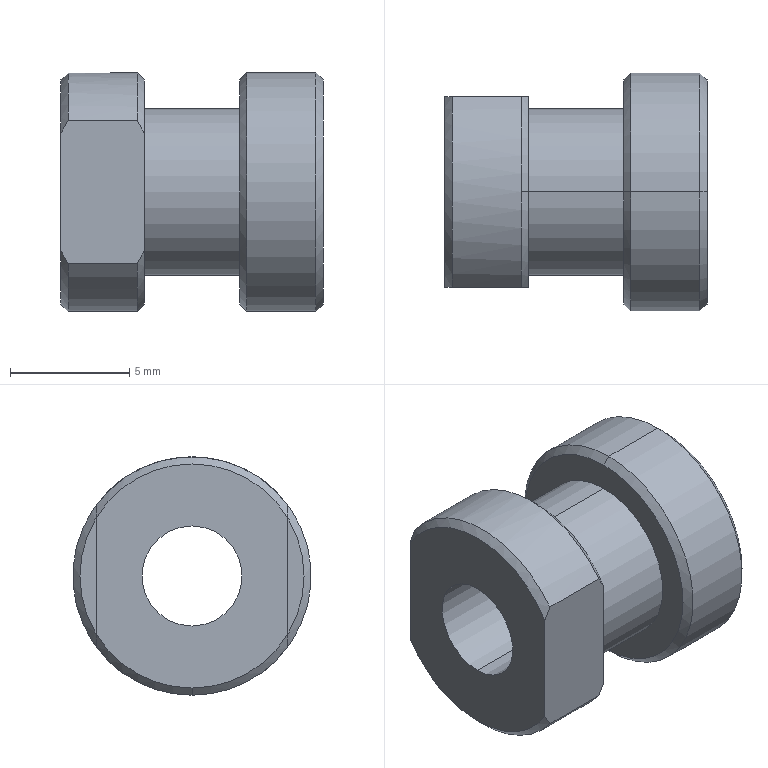Part | NX | features BREP 1 | 1 solid | 25 faces | box 11 x 10 x 10 mm | volume 518.249 mm3 | cone 10 | cylinder 9 | plane 6 | commonest cylinder face diameters 10 x5 4.2 x2 7 x2
STEP:
#1=CARTESIAN_POINT('',(7.5,0.,-2.1));
#2=VERTEX_POINT('',#1);
#3=CARTESIAN_POINT('',(7.5,0.,2.1));
#4=VERTEX_POINT('',#3);
#5=CARTESIAN_POINT('',(7.5,0.,0.));
#6=DIRECTION('',(-1.,0.,0.));
#7=DIRECTION('',(0.,0.,1.));
#8=AXIS2_PLACEMENT_3D('',#5,#6,#7);
#9=CIRCLE('',#8,2.1);
#10=EDGE_CURVE('',#2,#4,#9,.T.);
#11=ORIENTED_EDGE('',*,*,#10,.F.);
#12=CARTESIAN_POINT('',(-3.5,0.,-2.1));
#13=VERTEX_POINT('',#12);
#14=CARTESIAN_POINT('',(-3.5,0.,-2.1));
#15=DIRECTION('',(-1.,0.,0.));
#16=VECTOR('',#15,1000.);
#17=LINE('',#14,#16);
#18=EDGE_CURVE('',#13,#2,#17,.F.);
#19=ORIENTED_EDGE('',*,*,#18,.F.);
#20=CARTESIAN_POINT('',(-3.5,0.,2.1));
#21=VERTEX_POINT('',#20);
#22=CARTESIAN_POINT('',(-3.5,0.,0.));
#23=DIRECTION('',(-1.,0.,0.));
#24=DIRECTION('',(0.,0.,1.));
#25=AXIS2_PLACEMENT_3D('',#22,#23,#24);
#26=CIRCLE('',#25,2.1);
#27=EDGE_CURVE('',#13,#21,#26,.T.);
#28=ORIENTED_EDGE('',*,*,#27,.T.);
#29=CARTESIAN_POINT('',(-3.5,0.,2.1));
#30=DIRECTION('',(-1.,0.,0.));
#31=VECTOR('',#30,1000.);
#32=LINE('',#29,#31);
#33=EDGE_CURVE('',#21,#4,#32,.F.);
#34=ORIENTED_EDGE('',*,*,#33,.T.);
#35=EDGE_LOOP('',(#11,#19,#28,#34));
#36=FACE_BOUND('',#35,.T.);
#37=CARTESIAN_POINT('',(-3.5,0.,0.));
#38=DIRECTION('',(-1.,0.,0.));
#39=DIRECTION('',(0.,0.,1.));
#40=AXIS2_PLACEMENT_3D('',#37,#38,#39);
#41=CYLINDRICAL_SURFACE('',#40,2.1);
#42=ADVANCED_FACE('',(#36),#41,.F.);
#43=CARTESIAN_POINT('',(4.,0.,4.7));
#44=VERTEX_POINT('',#43);
#45=CARTESIAN_POINT('',(4.,0.,-4.7));
#46=VERTEX_POINT('',#45);
#47=CARTESIAN_POINT('',(4.,0.,0.));
#48=DIRECTION('',(-1.,0.,0.));
#49=DIRECTION('',(0.,0.,1.));
#50=AXIS2_PLACEMENT_3D('',#47,#48,#49);
#51=CIRCLE('',#50,4.7);
#52=EDGE_CURVE('',#44,#46,#51,.T.);
#53=ORIENTED_EDGE('',*,*,#52,.F.);
#54=CARTESIAN_POINT('',(4.3,0.,5.));
#55=VERTEX_POINT('',#54);
#56=CARTESIAN_POINT('',(4.3,0.,5.));
#57=DIRECTION('',(0.7071,0.,0.7071));
#58=VECTOR('',#57,1000.);
#59=LINE('',#56,#58);
#60=EDGE_CURVE('',#44,#55,#59,.T.);
#61=ORIENTED_EDGE('',*,*,#60,.T.);
#62=CARTESIAN_POINT('',(4.3,0.,-5.));
#63=VERTEX_POINT('',#62);
#64=CARTESIAN_POINT('',(4.3,0.,0.));
#65=DIRECTION('',(1.,0.,0.));
#66=DIRECTION('',(0.,0.,1.));
#67=AXIS2_PLACEMENT_3D('',#64,#65,#66);
#68=CIRCLE('',#67,5.);
#69=EDGE_CURVE('',#63,#55,#68,.T.);
#70=ORIENTED_EDGE('',*,*,#69,.F.);
#71=CARTESIAN_POINT('',(4.3,0.,-5.));
#72=DIRECTION('',(0.7071,0.,-0.7071));
#73=VECTOR('',#72,1000.);
#74=LINE('',#71,#73);
#75=EDGE_CURVE('',#46,#63,#74,.T.);
#76=ORIENTED_EDGE('',*,*,#75,.F.);
#77=EDGE_LOOP('',(#53,#61,#70,#76));
#78=FACE_BOUND('',#77,.T.);
#79=CARTESIAN_POINT('',(4.3,0.,0.));
#80=DIRECTION('',(1.,0.,0.));
#81=DIRECTION('',(0.,0.,-1.));
#82=AXIS2_PLACEMENT_3D('',#79,#80,#81);
#83=CONICAL_SURFACE('',#82,5.,0.7854);
#84=ADVANCED_FACE('',(#78),#83,.T.);
#85=CARTESIAN_POINT('',(7.5,0.,-4.7));
#86=VERTEX_POINT('',#85);
#87=CARTESIAN_POINT('',(7.5,0.,4.7));
#88=VERTEX_POINT('',#87);
#89=CARTESIAN_POINT('',(7.5,0.,0.));
#90=DIRECTION('',(1.,0.,0.));
#91=DIRECTION('',(0.,0.,-1.));
#92=AXIS2_PLACEMENT_3D('',#89,#90,#91);
#93=CIRCLE('',#92,4.7);
#94=EDGE_CURVE('',#86,#88,#93,.T.);
#95=ORIENTED_EDGE('',*,*,#94,.F.);
#96=CARTESIAN_POINT('',(7.2,0.,-5.));
#97=VERTEX_POINT('',#96);
#98=CARTESIAN_POINT('',(7.5,0.,-4.7));
#99=DIRECTION('',(-0.7071,0.,-0.7071));
#100=VECTOR('',#99,1000.);
#101=LINE('',#98,#100);
#102=EDGE_CURVE('',#97,#86,#101,.F.);
#103=ORIENTED_EDGE('',*,*,#102,.F.);
#104=CARTESIAN_POINT('',(7.2,0.,5.));
#105=VERTEX_POINT('',#104);
#106=CARTESIAN_POINT('',(7.2,0.,0.));
#107=DIRECTION('',(-1.,0.,0.));
#108=DIRECTION('',(0.,0.,-1.));
#109=AXIS2_PLACEMENT_3D('',#106,#107,#108);
#110=CIRCLE('',#109,5.);
#111=EDGE_CURVE('',#105,#97,#110,.T.);
#112=ORIENTED_EDGE('',*,*,#111,.F.);
#113=CARTESIAN_POINT('',(7.5,0.,4.7));
#114=DIRECTION('',(-0.7071,0.,0.7071));
#115=VECTOR('',#114,1000.);
#116=LINE('',#113,#115);
#117=EDGE_CURVE('',#105,#88,#116,.F.);
#118=ORIENTED_EDGE('',*,*,#117,.T.);
#119=EDGE_LOOP('',(#95,#103,#112,#118));
#120=FACE_BOUND('',#119,.T.);
#121=CARTESIAN_POINT('',(7.5,0.,0.));
#122=DIRECTION('',(-1.,0.,0.));
#123=DIRECTION('',(0.,0.,1.));
#124=AXIS2_PLACEMENT_3D('',#121,#122,#123);
#125=CONICAL_SURFACE('',#124,4.7,0.7854);
#126=ADVANCED_FACE('',(#120),#125,.T.);
#127=CARTESIAN_POINT('',(0.,0.,-3.5));
#128=VERTEX_POINT('',#127);
#129=CARTESIAN_POINT('',(0.,0.,3.5));
#130=VERTEX_POINT('',#129);
#131=CARTESIAN_POINT('',(0.,0.,0.));
#132=DIRECTION('',(1.,0.,0.));
#133=DIRECTION('',(0.,0.,-1.));
#134=AXIS2_PLACEMENT_3D('',#131,#132,#133);
#135=CIRCLE('',#134,3.5);
#136=EDGE_CURVE('',#128,#130,#135,.T.);
#137=ORIENTED_EDGE('',*,*,#136,.T.);
#138=CARTESIAN_POINT('',(4.,0.,3.5));
#139=VERTEX_POINT('',#138);
#140=CARTESIAN_POINT('',(-9.2,0.,3.5));
#141=DIRECTION('',(1.,0.,0.));
#142=VECTOR('',#141,1000.);
#143=LINE('',#140,#142);
#144=EDGE_CURVE('',#130,#139,#143,.T.);
#145=ORIENTED_EDGE('',*,*,#144,.T.);
#146=CARTESIAN_POINT('',(4.,0.,-3.5));
#147=VERTEX_POINT('',#146);
#148=CARTESIAN_POINT('',(4.,0.,0.));
#149=DIRECTION('',(1.,0.,0.));
#150=DIRECTION('',(0.,0.,-1.));
#151=AXIS2_PLACEMENT_3D('',#148,#149,#150);
#152=CIRCLE('',#151,3.5);
#153=EDGE_CURVE('',#147,#139,#152,.T.);
#154=ORIENTED_EDGE('',*,*,#153,.F.);
#155=CARTESIAN_POINT('',(-9.2,0.,-3.5));
#156=DIRECTION('',(1.,0.,0.));
#157=VECTOR('',#156,1000.);
#158=LINE('',#155,#157);
#159=EDGE_CURVE('',#128,#147,#158,.T.);
#160=ORIENTED_EDGE('',*,*,#159,.F.);
#161=EDGE_LOOP('',(#137,#145,#154,#160));
#162=FACE_BOUND('',#161,.T.);
#163=CARTESIAN_POINT('',(-9.2,0.,0.));
#164=DIRECTION('',(1.,0.,0.));
#165=DIRECTION('',(0.,0.,-1.));
#166=AXIS2_PLACEMENT_3D('',#163,#164,#165);
#167=CYLINDRICAL_SURFACE('',#166,3.5);
#168=ADVANCED_FACE('',(#162),#167,.T.);
#169=ORIENTED_EDGE('',*,*,#69,.T.);
#170=CARTESIAN_POINT('',(-9.2,0.,5.));
#171=DIRECTION('',(1.,0.,0.));
#172=VECTOR('',#171,1000.);
#173=LINE('',#170,#172);
#174=EDGE_CURVE('',#55,#105,#173,.T.);
#175=ORIENTED_EDGE('',*,*,#174,.T.);
#176=ORIENTED_EDGE('',*,*,#111,.T.);
#177=CARTESIAN_POINT('',(-9.2,0.,-5.));
#178=DIRECTION('',(1.,0.,0.));
#179=VECTOR('',#178,1000.);
#180=LINE('',#177,#179);
#181=EDGE_CURVE('',#63,#97,#180,.T.);
#182=ORIENTED_EDGE('',*,*,#181,.F.);
#183=EDGE_LOOP('',(#169,#175,#176,#182));
#184=FACE_BOUND('',#183,.T.);
#185=CARTESIAN_POINT('',(-9.2,0.,0.));
#186=DIRECTION('',(1.,0.,0.));
#187=DIRECTION('',(0.,0.,-1.));
#188=AXIS2_PLACEMENT_3D('',#185,#186,#187);
#189=CYLINDRICAL_SURFACE('',#188,5.);
#190=ADVANCED_FACE('',(#184),#189,.T.);
#191=CARTESIAN_POINT('',(-3.5,0.,-4.7));
#192=VERTEX_POINT('',#191);
#193=CARTESIAN_POINT('',(-3.5,-4.,-2.468));
#194=VERTEX_POINT('',#193);
#195=CARTESIAN_POINT('',(-3.5,0.,0.));
#196=DIRECTION('',(-1.,0.,0.));
#197=DIRECTION('',(0.,0.,1.));
#198=AXIS2_PLACEMENT_3D('',#195,#196,#197);
#199=CIRCLE('',#198,4.7);
#200=EDGE_CURVE('',#192,#194,#199,.T.);
#201=ORIENTED_EDGE('',*,*,#200,.F.);
#202=CARTESIAN_POINT('',(-3.2,0.,-5.));
#203=VERTEX_POINT('',#202);
#204=CARTESIAN_POINT('',(-3.2,0.,-5.));
#205=DIRECTION('',(0.7071,0.,-0.7071));
#206=VECTOR('',#205,1000.);
#207=LINE('',#204,#206);
#208=EDGE_CURVE('',#192,#203,#207,.T.);
#209=ORIENTED_EDGE('',*,*,#208,.T.);
#210=CARTESIAN_POINT('',(-3.2,-4.,-3.));
#211=VERTEX_POINT('',#210);
#212=CARTESIAN_POINT('',(-3.2,0.,0.));
#213=DIRECTION('',(1.,0.,0.));
#214=DIRECTION('',(0.,0.,1.));
#215=AXIS2_PLACEMENT_3D('',#212,#213,#214);
#216=CIRCLE('',#215,5.);
#217=EDGE_CURVE('',#211,#203,#216,.T.);
#218=ORIENTED_EDGE('',*,*,#217,.F.);
#219=CARTESIAN_POINT('',(-3.2,-4.,-3.));
#220=CARTESIAN_POINT('',(-3.305,-4.,-2.825));
#221=CARTESIAN_POINT('',(-3.405,-4.,-2.648));
#222=CARTESIAN_POINT('',(-3.5,-4.,-2.468));
#223=B_SPLINE_CURVE_WITH_KNOTS('',3,(#219,#220,#221,#222),.UNSPECIFIED.,.F.,.F.,(4,4),(0.009427,0.01004),.UNSPECIFIED.);
#224=EDGE_CURVE('',#211,#194,#223,.T.);
#225=ORIENTED_EDGE('',*,*,#224,.T.);
#226=EDGE_LOOP('',(#201,#209,#218,#225));
#227=FACE_BOUND('',#226,.T.);
#228=CARTESIAN_POINT('',(-3.2,0.,0.));
#229=DIRECTION('',(1.,0.,0.));
#230=DIRECTION('',(0.,0.,-1.));
#231=AXIS2_PLACEMENT_3D('',#228,#229,#230);
#232=CONICAL_SURFACE('',#231,5.,0.7854);
#233=ADVANCED_FACE('',(#227),#232,.T.);
#234=CARTESIAN_POINT('',(0.,0.,4.7));
#235=VERTEX_POINT('',#234);
#236=CARTESIAN_POINT('',(0.,-4.,2.468));
#237=VERTEX_POINT('',#236);
#238=CARTESIAN_POINT('',(0.,0.,0.));
#239=DIRECTION('',(1.,0.,0.));
#240=DIRECTION('',(0.,0.,-1.));
#241=AXIS2_PLACEMENT_3D('',#238,#239,#240);
#242=CIRCLE('',#241,4.7);
#243=EDGE_CURVE('',#235,#237,#242,.T.);
#244=ORIENTED_EDGE('',*,*,#243,.F.);
#245=CARTESIAN_POINT('',(-0.3,0.,5.));
#246=VERTEX_POINT('',#245);
#247=CARTESIAN_POINT('',(0.,0.,4.7));
#248=DIRECTION('',(-0.7071,0.,0.7071));
#249=VECTOR('',#248,1000.);
#250=LINE('',#247,#249);
#251=EDGE_CURVE('',#235,#246,#250,.T.);
#252=ORIENTED_EDGE('',*,*,#251,.T.);
#253=CARTESIAN_POINT('',(-0.3,-4.,3.));
#254=VERTEX_POINT('',#253);
#255=CARTESIAN_POINT('',(-0.3,0.,0.));
#256=DIRECTION('',(-1.,0.,0.));
#257=DIRECTION('',(0.,0.,-1.));
#258=AXIS2_PLACEMENT_3D('',#255,#256,#257);
#259=CIRCLE('',#258,5.);
#260=EDGE_CURVE('',#254,#246,#259,.T.);
#261=ORIENTED_EDGE('',*,*,#260,.F.);
#262=CARTESIAN_POINT('',(-0.3,-4.,3.));
#263=CARTESIAN_POINT('',(-0.195,-4.,2.825));
#264=CARTESIAN_POINT('',(-0.09455,-4.,2.648));
#265=CARTESIAN_POINT('',(0.,-4.,2.468));
#266=B_SPLINE_CURVE_WITH_KNOTS('',3,(#262,#263,#264,#265),.UNSPECIFIED.,.F.,.F.,(4,4),(0.009427,0.01004),.UNSPECIFIED.);
#267=EDGE_CURVE('',#254,#237,#266,.T.);
#268=ORIENTED_EDGE('',*,*,#267,.T.);
#269=EDGE_LOOP('',(#244,#252,#261,#268));
#270=FACE_BOUND('',#269,.T.);
#271=CARTESIAN_POINT('',(0.,0.,0.));
#272=DIRECTION('',(-1.,0.,0.));
#273=DIRECTION('',(0.,0.,1.));
#274=AXIS2_PLACEMENT_3D('',#271,#272,#273);
#275=CONICAL_SURFACE('',#274,4.7,0.7854);
#276=ADVANCED_FACE('',(#270),#275,.T.);
#277=ORIENTED_EDGE('',*,*,#217,.T.);
#278=CARTESIAN_POINT('',(-0.3,0.,-5.));
#279=VERTEX_POINT('',#278);
#280=CARTESIAN_POINT('',(-9.2,0.,-5.));
#281=DIRECTION('',(1.,0.,0.));
#282=VECTOR('',#281,1000.);
#283=LINE('',#280,#282);
#284=EDGE_CURVE('',#203,#279,#283,.T.);
#285=ORIENTED_EDGE('',*,*,#284,.T.);
#286=CARTESIAN_POINT('',(-0.3,-4.,-3.));
#287=VERTEX_POINT('',#286);
#288=CARTESIAN_POINT('',(-0.3,0.,0.));
#289=DIRECTION('',(-1.,0.,0.));
#290=DIRECTION('',(0.,0.,-1.));
#291=AXIS2_PLACEMENT_3D('',#288,#289,#290);
#292=CIRCLE('',#291,5.);
#293=EDGE_CURVE('',#279,#287,#292,.T.);
#294=ORIENTED_EDGE('',*,*,#293,.T.);
#295=CARTESIAN_POINT('',(-9.2,-4.,-3.));
#296=DIRECTION('',(-1.,0.,0.));
#297=VECTOR('',#296,1000.);
#298=LINE('',#295,#297);
#299=EDGE_CURVE('',#287,#211,#298,.T.);
#300=ORIENTED_EDGE('',*,*,#299,.T.);
#301=EDGE_LOOP('',(#277,#285,#294,#300));
#302=FACE_BOUND('',#301,.T.);
#303=CARTESIAN_POINT('',(-9.2,0.,0.));
#304=DIRECTION('',(1.,0.,0.));
#305=DIRECTION('',(0.,0.,-1.));
#306=AXIS2_PLACEMENT_3D('',#303,#304,#305);
#307=CYLINDRICAL_SURFACE('',#306,5.);
#308=ADVANCED_FACE('',(#302),#307,.T.);
#309=CARTESIAN_POINT('',(0.,-4.,-2.468));
#310=VERTEX_POINT('',#309);
#311=CARTESIAN_POINT('',(0.,4.,-2.468));
#312=VERTEX_POINT('',#311);
#313=CARTESIAN_POINT('',(0.,0.,0.));
#314=DIRECTION('',(1.,0.,0.));
#315=DIRECTION('',(0.,0.,-1.));
#316=AXIS2_PLACEMENT_3D('',#313,#314,#315);
#317=CIRCLE('',#316,4.7);
#318=EDGE_CURVE('',#310,#312,#317,.T.);
#319=ORIENTED_EDGE('',*,*,#318,.T.);
#320=CARTESIAN_POINT('',(0.,4.,2.468));
#321=VERTEX_POINT('',#320);
#322=CARTESIAN_POINT('',(0.,4.,-8.));
#323=DIRECTION('',(0.,0.,-1.));
#324=VECTOR('',#323,1000.);
#325=LINE('',#322,#324);
#326=EDGE_CURVE('',#321,#312,#325,.T.);
#327=ORIENTED_EDGE('',*,*,#326,.F.);
#328=CARTESIAN_POINT('',(0.,0.,0.));
#329=DIRECTION('',(1.,0.,0.));
#330=DIRECTION('',(0.,0.,-1.));
#331=AXIS2_PLACEMENT_3D('',#328,#329,#330);
#332=CIRCLE('',#331,4.7);
#333=EDGE_CURVE('',#321,#235,#332,.T.);
#334=ORIENTED_EDGE('',*,*,#333,.T.);
#335=ORIENTED_EDGE('',*,*,#243,.T.);
#336=CARTESIAN_POINT('',(0.,-4.,-8.));
#337=DIRECTION('',(0.,0.,1.));
#338=VECTOR('',#337,1000.);
#339=LINE('',#336,#338);
#340=EDGE_CURVE('',#310,#237,#339,.T.);
#341=ORIENTED_EDGE('',*,*,#340,.F.);
#342=EDGE_LOOP('',(#319,#327,#334,#335,#341));
#343=FACE_BOUND('',#342,.T.);
#344=ORIENTED_EDGE('',*,*,#136,.F.);
#345=CARTESIAN_POINT('',(0.,0.,0.));
#346=DIRECTION('',(1.,0.,0.));
#347=DIRECTION('',(0.,0.,-1.));
#348=AXIS2_PLACEMENT_3D('',#345,#346,#347);
#349=CIRCLE('',#348,3.5);
#350=EDGE_CURVE('',#130,#128,#349,.T.);
#351=ORIENTED_EDGE('',*,*,#350,.F.);
#352=EDGE_LOOP('',(#344,#351));
#353=FACE_BOUND('',#352,.T.);
#354=CARTESIAN_POINT('',(0.,5.,0.));
#355=DIRECTION('',(1.,0.,0.));
#356=DIRECTION('',(0.,1.,0.));
#357=AXIS2_PLACEMENT_3D('',#354,#355,#356);
#358=PLANE('',#357);
#359=ADVANCED_FACE('',(#343,#353),#358,.T.);
#360=ORIENTED_EDGE('',*,*,#260,.T.);
#361=CARTESIAN_POINT('',(-0.3,4.,3.));
#362=VERTEX_POINT('',#361);
#363=CARTESIAN_POINT('',(-0.3,0.,0.));
#364=DIRECTION('',(-1.,0.,0.));
#365=DIRECTION('',(0.,0.,-1.));
#366=AXIS2_PLACEMENT_3D('',#363,#364,#365);
#367=CIRCLE('',#366,5.);
#368=EDGE_CURVE('',#246,#362,#367,.T.);
#369=ORIENTED_EDGE('',*,*,#368,.T.);
#370=CARTESIAN_POINT('',(-3.2,4.,3.));
#371=VERTEX_POINT('',#370);
#372=CARTESIAN_POINT('',(-9.2,4.,3.));
#373=DIRECTION('',(-1.,0.,0.));
#374=VECTOR('',#373,1000.);
#375=LINE('',#372,#374);
#376=EDGE_CURVE('',#362,#371,#375,.T.);
#377=ORIENTED_EDGE('',*,*,#376,.T.);
#378=CARTESIAN_POINT('',(-3.2,-4.,3.));
#379=VERTEX_POINT('',#378);
#380=CARTESIAN_POINT('',(-3.2,0.,0.));
#381=DIRECTION('',(1.,0.,0.));
#382=DIRECTION('',(0.,0.,1.));
#383=AXIS2_PLACEMENT_3D('',#380,#381,#382);
#384=CIRCLE('',#383,5.);
#385=EDGE_CURVE('',#371,#379,#384,.T.);
#386=ORIENTED_EDGE('',*,*,#385,.T.);
#387=CARTESIAN_POINT('',(-9.2,-4.,3.));
#388=DIRECTION('',(1.,0.,0.));
#389=VECTOR('',#388,1000.);
#390=LINE('',#387,#389);
#391=EDGE_CURVE('',#379,#254,#390,.T.);
#392=ORIENTED_EDGE('',*,*,#391,.T.);
#393=EDGE_LOOP('',(#360,#369,#377,#386,#392));
#394=FACE_BOUND('',#393,.T.);
#395=CARTESIAN_POINT('',(-9.2,0.,0.));
#396=DIRECTION('',(1.,0.,0.));
#397=DIRECTION('',(0.,0.,-1.));
#398=AXIS2_PLACEMENT_3D('',#395,#396,#397);
#399=CYLINDRICAL_SURFACE('',#398,5.);
#400=ADVANCED_FACE('',(#394),#399,.T.);
#401=ORIENTED_EDGE('',*,*,#284,.F.);
#402=CARTESIAN_POINT('',(-3.2,4.,-3.));
#403=VERTEX_POINT('',#402);
#404=CARTESIAN_POINT('',(-3.2,0.,0.));
#405=DIRECTION('',(1.,0.,0.));
#406=DIRECTION('',(0.,0.,1.));
#407=AXIS2_PLACEMENT_3D('',#404,#405,#406);
#408=CIRCLE('',#407,5.);
#409=EDGE_CURVE('',#203,#403,#408,.T.);
#410=ORIENTED_EDGE('',*,*,#409,.T.);
#411=CARTESIAN_POINT('',(-0.3,4.,-3.));
#412=VERTEX_POINT('',#411);
#413=CARTESIAN_POINT('',(-9.2,4.,-3.));
#414=DIRECTION('',(1.,0.,0.));
#415=VECTOR('',#414,1000.);
#416=LINE('',#413,#415);
#417=EDGE_CURVE('',#403,#412,#416,.T.);
#418=ORIENTED_EDGE('',*,*,#417,.T.);
#419=CARTESIAN_POINT('',(-0.3,0.,0.));
#420=DIRECTION('',(-1.,0.,0.));
#421=DIRECTION('',(0.,0.,-1.));
#422=AXIS2_PLACEMENT_3D('',#419,#420,#421);
#423=CIRCLE('',#422,5.);
#424=EDGE_CURVE('',#412,#279,#423,.T.);
#425=ORIENTED_EDGE('',*,*,#424,.T.);
#426=EDGE_LOOP('',(#401,#410,#418,#425));
#427=FACE_BOUND('',#426,.T.);
#428=CARTESIAN_POINT('',(-9.2,0.,0.));
#429=DIRECTION('',(1.,0.,0.));
#430=DIRECTION('',(0.,0.,-1.));
#431=AXIS2_PLACEMENT_3D('',#428,#429,#430);
#432=CYLINDRICAL_SURFACE('',#431,5.);
#433=ADVANCED_FACE('',(#427),#432,.T.);
#434=CARTESIAN_POINT('',(-3.5,-4.,2.468));
#435=VERTEX_POINT('',#434);
#436=CARTESIAN_POINT('',(-3.5,4.,2.468));
#437=VERTEX_POINT('',#436);
#438=CARTESIAN_POINT('',(-3.5,0.,0.));
#439=DIRECTION('',(-1.,0.,0.));
#440=DIRECTION('',(0.,0.,1.));
#441=AXIS2_PLACEMENT_3D('',#438,#439,#440);
#442=CIRCLE('',#441,4.7);
#443=EDGE_CURVE('',#435,#437,#442,.T.);
#444=ORIENTED_EDGE('',*,*,#443,.T.);
#445=CARTESIAN_POINT('',(-3.5,4.,-2.468));
#446=VERTEX_POINT('',#445);
#447=CARTESIAN_POINT('',(-3.5,4.,-8.));
#448=DIRECTION('',(0.,0.,-1.));
#449=VECTOR('',#448,1000.);
#450=LINE('',#447,#449);
#451=EDGE_CURVE('',#437,#446,#450,.T.);
#452=ORIENTED_EDGE('',*,*,#451,.T.);
#453=CARTESIAN_POINT('',(-3.5,0.,0.));
#454=DIRECTION('',(-1.,0.,0.));
#455=DIRECTION('',(0.,0.,1.));
#456=AXIS2_PLACEMENT_3D('',#453,#454,#455);
#457=CIRCLE('',#456,4.7);
#458=EDGE_CURVE('',#446,#192,#457,.T.);
#459=ORIENTED_EDGE('',*,*,#458,.T.);
#460=ORIENTED_EDGE('',*,*,#200,.T.);
#461=CARTESIAN_POINT('',(-3.5,-4.,-8.));
#462=DIRECTION('',(0.,0.,1.));
#463=VECTOR('',#462,1000.);
#464=LINE('',#461,#463);
#465=EDGE_CURVE('',#194,#435,#464,.T.);
#466=ORIENTED_EDGE('',*,*,#465,.T.);
#467=EDGE_LOOP('',(#444,#452,#459,#460,#466));
#468=FACE_BOUND('',#467,.T.);
#469=CARTESIAN_POINT('',(-3.5,0.,0.));
#470=DIRECTION('',(-1.,0.,0.));
#471=DIRECTION('',(0.,0.,1.));
#472=AXIS2_PLACEMENT_3D('',#469,#470,#471);
#473=CIRCLE('',#472,2.1);
#474=EDGE_CURVE('',#21,#13,#473,.T.);
#475=ORIENTED_EDGE('',*,*,#474,.F.);
#476=ORIENTED_EDGE('',*,*,#27,.F.);
#477=EDGE_LOOP('',(#475,#476));
#478=FACE_BOUND('',#477,.T.);
#479=CARTESIAN_POINT('',(-3.5,0.,0.));
#480=DIRECTION('',(-1.,0.,0.));
#481=DIRECTION('',(0.,0.,1.));
#482=AXIS2_PLACEMENT_3D('',#479,#480,#481);
#483=PLANE('',#482);
#484=ADVANCED_FACE('',(#468,#478),#483,.T.);
#485=ORIENTED_EDGE('',*,*,#424,.F.);
#486=CARTESIAN_POINT('',(-0.3,4.,-3.));
#487=CARTESIAN_POINT('',(-0.195,4.,-2.825));
#488=CARTESIAN_POINT('',(-0.09455,4.,-2.648));
#489=CARTESIAN_POINT('',(0.,4.,-2.468));
#490=B_SPLINE_CURVE_WITH_KNOTS('',3,(#486,#487,#488,#489),.UNSPECIFIED.,.F.,.F.,(4,4),(0.009427,0.01004),.UNSPECIFIED.);
#491=EDGE_CURVE('',#412,#312,#490,.T.);
#492=ORIENTED_EDGE('',*,*,#491,.T.);
#493=ORIENTED_EDGE('',*,*,#318,.F.);
#494=CARTESIAN_POINT('',(0.,-4.,-2.468));
#495=CARTESIAN_POINT('',(-0.09472,-4.,-2.648));
#496=CARTESIAN_POINT('',(-0.1952,-4.,-2.825));
#497=CARTESIAN_POINT('',(-0.3,-4.,-3.));
#498=B_SPLINE_CURVE_WITH_KNOTS('',3,(#494,#495,#496,#497),.UNSPECIFIED.,.F.,.F.,(4,4),(0.01523,0.01584),.UNSPECIFIED.);
#499=EDGE_CURVE('',#310,#287,#498,.T.);
#500=ORIENTED_EDGE('',*,*,#499,.T.);
#501=ORIENTED_EDGE('',*,*,#293,.F.);
#502=EDGE_LOOP('',(#485,#492,#493,#500,#501));
#503=FACE_BOUND('',#502,.T.);
#504=CARTESIAN_POINT('',(0.,0.,0.));
#505=DIRECTION('',(-1.,0.,0.));
#506=DIRECTION('',(0.,0.,1.));
#507=AXIS2_PLACEMENT_3D('',#504,#505,#506);
#508=CONICAL_SURFACE('',#507,4.7,0.7854);
#509=ADVANCED_FACE('',(#503),#508,.T.);
#510=ORIENTED_EDGE('',*,*,#251,.F.);
#511=ORIENTED_EDGE('',*,*,#333,.F.);
#512=CARTESIAN_POINT('',(0.,4.,2.468));
#513=CARTESIAN_POINT('',(-0.09472,4.,2.648));
#514=CARTESIAN_POINT('',(-0.1952,4.,2.825));
#515=CARTESIAN_POINT('',(-0.3,4.,3.));
#516=B_SPLINE_CURVE_WITH_KNOTS('',3,(#512,#513,#514,#515),.UNSPECIFIED.,.F.,.F.,(4,4),(0.01523,0.01584),.UNSPECIFIED.);
#517=EDGE_CURVE('',#321,#362,#516,.T.);
#518=ORIENTED_EDGE('',*,*,#517,.T.);
#519=ORIENTED_EDGE('',*,*,#368,.F.);
#520=EDGE_LOOP('',(#510,#511,#518,#519));
#521=FACE_BOUND('',#520,.T.);
#522=CARTESIAN_POINT('',(0.,0.,0.));
#523=DIRECTION('',(-1.,0.,0.));
#524=DIRECTION('',(0.,0.,1.));
#525=AXIS2_PLACEMENT_3D('',#522,#523,#524);
#526=CONICAL_SURFACE('',#525,4.7,0.7854);
#527=ADVANCED_FACE('',(#521),#526,.T.);
#528=ORIENTED_EDGE('',*,*,#385,.F.);
#529=CARTESIAN_POINT('',(-3.2,4.,3.));
#530=CARTESIAN_POINT('',(-3.305,4.,2.825));
#531=CARTESIAN_POINT('',(-3.405,4.,2.648));
#532=CARTESIAN_POINT('',(-3.5,4.,2.468));
#533=B_SPLINE_CURVE_WITH_KNOTS('',3,(#529,#530,#531,#532),.UNSPECIFIED.,.F.,.F.,(4,4),(0.009427,0.01004),.UNSPECIFIED.);
#534=EDGE_CURVE('',#371,#437,#533,.T.);
#535=ORIENTED_EDGE('',*,*,#534,.T.);
#536=ORIENTED_EDGE('',*,*,#443,.F.);
#537=CARTESIAN_POINT('',(-3.5,-4.,2.468));
#538=CARTESIAN_POINT('',(-3.405,-4.,2.648));
#539=CARTESIAN_POINT('',(-3.305,-4.,2.825));
#540=CARTESIAN_POINT('',(-3.2,-4.,3.));
#541=B_SPLINE_CURVE_WITH_KNOTS('',3,(#537,#538,#539,#540),.UNSPECIFIED.,.F.,.F.,(4,4),(0.01523,0.01584),.UNSPECIFIED.);
#542=EDGE_CURVE('',#435,#379,#541,.T.);
#543=ORIENTED_EDGE('',*,*,#542,.T.);
#544=EDGE_LOOP('',(#528,#535,#536,#543));
#545=FACE_BOUND('',#544,.T.);
#546=CARTESIAN_POINT('',(-3.2,0.,0.));
#547=DIRECTION('',(1.,0.,0.));
#548=DIRECTION('',(0.,0.,-1.));
#549=AXIS2_PLACEMENT_3D('',#546,#547,#548);
#550=CONICAL_SURFACE('',#549,5.,0.7854);
#551=ADVANCED_FACE('',(#545),#550,.T.);
#552=ORIENTED_EDGE('',*,*,#208,.F.);
#553=ORIENTED_EDGE('',*,*,#458,.F.);
#554=CARTESIAN_POINT('',(-3.5,4.,-2.468));
#555=CARTESIAN_POINT('',(-3.405,4.,-2.648));
#556=CARTESIAN_POINT('',(-3.305,4.,-2.825));
#557=CARTESIAN_POINT('',(-3.2,4.,-3.));
#558=B_SPLINE_CURVE_WITH_KNOTS('',3,(#554,#555,#556,#557),.UNSPECIFIED.,.F.,.F.,(4,4),(0.01523,0.01584),.UNSPECIFIED.);
#559=EDGE_CURVE('',#446,#403,#558,.T.);
#560=ORIENTED_EDGE('',*,*,#559,.T.);
#561=ORIENTED_EDGE('',*,*,#409,.F.);
#562=EDGE_LOOP('',(#552,#553,#560,#561));
#563=FACE_BOUND('',#562,.T.);
#564=CARTESIAN_POINT('',(-3.2,0.,0.));
#565=DIRECTION('',(1.,0.,0.));
#566=DIRECTION('',(0.,0.,-1.));
#567=AXIS2_PLACEMENT_3D('',#564,#565,#566);
#568=CONICAL_SURFACE('',#567,5.,0.7854);
#569=ADVANCED_FACE('',(#563),#568,.T.);
#570=ORIENTED_EDGE('',*,*,#174,.F.);
#571=CARTESIAN_POINT('',(4.3,0.,0.));
#572=DIRECTION('',(1.,0.,0.));
#573=DIRECTION('',(0.,0.,1.));
#574=AXIS2_PLACEMENT_3D('',#571,#572,#573);
#575=CIRCLE('',#574,5.);
#576=EDGE_CURVE('',#55,#63,#575,.T.);
#577=ORIENTED_EDGE('',*,*,#576,.T.);
#578=ORIENTED_EDGE('',*,*,#181,.T.);
#579=CARTESIAN_POINT('',(7.2,0.,0.));
#580=DIRECTION('',(-1.,0.,0.));
#581=DIRECTION('',(0.,0.,-1.));
#582=AXIS2_PLACEMENT_3D('',#579,#580,#581);
#583=CIRCLE('',#582,5.);
#584=EDGE_CURVE('',#97,#105,#583,.T.);
#585=ORIENTED_EDGE('',*,*,#584,.T.);
#586=EDGE_LOOP('',(#570,#577,#578,#585));
#587=FACE_BOUND('',#586,.T.);
#588=CARTESIAN_POINT('',(-9.2,0.,0.));
#589=DIRECTION('',(1.,0.,0.));
#590=DIRECTION('',(0.,0.,-1.));
#591=AXIS2_PLACEMENT_3D('',#588,#589,#590);
#592=CYLINDRICAL_SURFACE('',#591,5.);
#593=ADVANCED_FACE('',(#587),#592,.T.);
#594=CARTESIAN_POINT('',(4.,0.,0.));
#595=DIRECTION('',(-1.,0.,0.));
#596=DIRECTION('',(0.,0.,1.));
#597=AXIS2_PLACEMENT_3D('',#594,#595,#596);
#598=CIRCLE('',#597,4.7);
#599=EDGE_CURVE('',#46,#44,#598,.T.);
#600=ORIENTED_EDGE('',*,*,#599,.T.);
#601=ORIENTED_EDGE('',*,*,#52,.T.);
#602=EDGE_LOOP('',(#600,#601));
#603=FACE_BOUND('',#602,.T.);
#604=ORIENTED_EDGE('',*,*,#153,.T.);
#605=CARTESIAN_POINT('',(4.,0.,0.));
#606=DIRECTION('',(1.,0.,0.));
#607=DIRECTION('',(0.,0.,-1.));
#608=AXIS2_PLACEMENT_3D('',#605,#606,#607);
#609=CIRCLE('',#608,3.5);
#610=EDGE_CURVE('',#139,#147,#609,.T.);
#611=ORIENTED_EDGE('',*,*,#610,.T.);
#612=EDGE_LOOP('',(#604,#611));
#613=FACE_BOUND('',#612,.T.);
#614=CARTESIAN_POINT('',(4.,5.,0.));
#615=DIRECTION('',(-1.,0.,0.));
#616=DIRECTION('',(0.,0.,1.));
#617=AXIS2_PLACEMENT_3D('',#614,#615,#616);
#618=PLANE('',#617);
#619=ADVANCED_FACE('',(#603,#613),#618,.T.);
#620=ORIENTED_EDGE('',*,*,#144,.F.);
#621=ORIENTED_EDGE('',*,*,#350,.T.);
#622=ORIENTED_EDGE('',*,*,#159,.T.);
#623=ORIENTED_EDGE('',*,*,#610,.F.);
#624=EDGE_LOOP('',(#620,#621,#622,#623));
#625=FACE_BOUND('',#624,.T.);
#626=CARTESIAN_POINT('',(-9.2,0.,0.));
#627=DIRECTION('',(1.,0.,0.));
#628=DIRECTION('',(0.,0.,-1.));
#629=AXIS2_PLACEMENT_3D('',#626,#627,#628);
#630=CYLINDRICAL_SURFACE('',#629,3.5);
#631=ADVANCED_FACE('',(#625),#630,.T.);
#632=CARTESIAN_POINT('',(7.5,0.,0.));
#633=DIRECTION('',(1.,0.,0.));
#634=DIRECTION('',(0.,0.,-1.));
#635=AXIS2_PLACEMENT_3D('',#632,#633,#634);
#636=CIRCLE('',#635,4.7);
#637=EDGE_CURVE('',#88,#86,#636,.T.);
#638=ORIENTED_EDGE('',*,*,#637,.T.);
#639=ORIENTED_EDGE('',*,*,#94,.T.);
#640=EDGE_LOOP('',(#638,#639));
#641=FACE_BOUND('',#640,.T.);
#642=CARTESIAN_POINT('',(7.5,0.,0.));
#643=DIRECTION('',(-1.,0.,0.));
#644=DIRECTION('',(0.,0.,1.));
#645=AXIS2_PLACEMENT_3D('',#642,#643,#644);
#646=CIRCLE('',#645,2.1);
#647=EDGE_CURVE('',#4,#2,#646,.T.);
#648=ORIENTED_EDGE('',*,*,#647,.T.);
#649=ORIENTED_EDGE('',*,*,#10,.T.);
#650=EDGE_LOOP('',(#648,#649));
#651=FACE_BOUND('',#650,.T.);
#652=CARTESIAN_POINT('',(7.5,0.,0.));
#653=DIRECTION('',(1.,0.,0.));
#654=DIRECTION('',(0.,1.,0.));
#655=AXIS2_PLACEMENT_3D('',#652,#653,#654);
#656=PLANE('',#655);
#657=ADVANCED_FACE('',(#641,#651),#656,.T.);
#658=ORIENTED_EDGE('',*,*,#102,.T.);
#659=ORIENTED_EDGE('',*,*,#637,.F.);
#660=ORIENTED_EDGE('',*,*,#117,.F.);
#661=ORIENTED_EDGE('',*,*,#584,.F.);
#662=EDGE_LOOP('',(#658,#659,#660,#661));
#663=FACE_BOUND('',#662,.T.);
#664=CARTESIAN_POINT('',(7.5,0.,0.));
#665=DIRECTION('',(-1.,0.,0.));
#666=DIRECTION('',(0.,0.,1.));
#667=AXIS2_PLACEMENT_3D('',#664,#665,#666);
#668=CONICAL_SURFACE('',#667,4.7,0.7854);
#669=ADVANCED_FACE('',(#663),#668,.T.);
#670=ORIENTED_EDGE('',*,*,#60,.F.);
#671=ORIENTED_EDGE('',*,*,#599,.F.);
#672=ORIENTED_EDGE('',*,*,#75,.T.);
#673=ORIENTED_EDGE('',*,*,#576,.F.);
#674=EDGE_LOOP('',(#670,#671,#672,#673));
#675=FACE_BOUND('',#674,.T.);
#676=CARTESIAN_POINT('',(4.3,0.,0.));
#677=DIRECTION('',(1.,0.,0.));
#678=DIRECTION('',(0.,0.,-1.));
#679=AXIS2_PLACEMENT_3D('',#676,#677,#678);
#680=CONICAL_SURFACE('',#679,5.,0.7854);
#681=ADVANCED_FACE('',(#675),#680,.T.);
#682=ORIENTED_EDGE('',*,*,#340,.T.);
#683=ORIENTED_EDGE('',*,*,#267,.F.);
#684=ORIENTED_EDGE('',*,*,#391,.F.);
#685=ORIENTED_EDGE('',*,*,#542,.F.);
#686=ORIENTED_EDGE('',*,*,#465,.F.);
#687=ORIENTED_EDGE('',*,*,#224,.F.);
#688=ORIENTED_EDGE('',*,*,#299,.F.);
#689=ORIENTED_EDGE('',*,*,#499,.F.);
#690=EDGE_LOOP('',(#682,#683,#684,#685,#686,#687,#688,#689));
#691=FACE_BOUND('',#690,.T.);
#692=CARTESIAN_POINT('',(19.057,-4.,-8.));
#693=DIRECTION('',(0.,-1.,0.));
#694=DIRECTION('',(0.,0.,-1.));
#695=AXIS2_PLACEMENT_3D('',#692,#693,#694);
#696=PLANE('',#695);
#697=ADVANCED_FACE('',(#691),#696,.T.);
#698=ORIENTED_EDGE('',*,*,#326,.T.);
#699=ORIENTED_EDGE('',*,*,#491,.F.);
#700=ORIENTED_EDGE('',*,*,#417,.F.);
#701=ORIENTED_EDGE('',*,*,#559,.F.);
#702=ORIENTED_EDGE('',*,*,#451,.F.);
#703=ORIENTED_EDGE('',*,*,#534,.F.);
#704=ORIENTED_EDGE('',*,*,#376,.F.);
#705=ORIENTED_EDGE('',*,*,#517,.F.);
#706=EDGE_LOOP('',(#698,#699,#700,#701,#702,#703,#704,#705));
#707=FACE_BOUND('',#706,.T.);
#708=CARTESIAN_POINT('',(19.057,4.,-8.));
#709=DIRECTION('',(0.,1.,0.));
#710=DIRECTION('',(1.,0.,0.));
#711=AXIS2_PLACEMENT_3D('',#708,#709,#710);
#712=PLANE('',#711);
#713=ADVANCED_FACE('',(#707),#712,.T.);
#714=ORIENTED_EDGE('',*,*,#18,.T.);
#715=ORIENTED_EDGE('',*,*,#647,.F.);
#716=ORIENTED_EDGE('',*,*,#33,.F.);
#717=ORIENTED_EDGE('',*,*,#474,.T.);
#718=EDGE_LOOP('',(#714,#715,#716,#717));
#719=FACE_BOUND('',#718,.T.);
#720=CARTESIAN_POINT('',(-3.5,0.,0.));
#721=DIRECTION('',(-1.,0.,0.));
#722=DIRECTION('',(0.,0.,1.));
#723=AXIS2_PLACEMENT_3D('',#720,#721,#722);
#724=CYLINDRICAL_SURFACE('',#723,2.1);
#725=ADVANCED_FACE('',(#719),#724,.F.);
#726=CLOSED_SHELL('',(#42,#84,#126,#168,#190,#233,#276,#308,#359,#400,#433,#484,#509,#527,#551,#569,#593,#619,#631,#657,#669,#681,#697,#713,#725));
#727=MANIFOLD_SOLID_BREP('',#726);
#728=(LENGTH_UNIT()NAMED_UNIT(*)SI_UNIT(.MILLI.,.METRE.));
#729=UNCERTAINTY_MEASURE_WITH_UNIT(LENGTH_MEASURE(0.00001),#728,'','');
#730=(NAMED_UNIT(*)PLANE_ANGLE_UNIT()SI_UNIT($,.RADIAN.));
#731=(NAMED_UNIT(*)SI_UNIT($,.STERADIAN.)SOLID_ANGLE_UNIT());
#732=(GEOMETRIC_REPRESENTATION_CONTEXT(3)GLOBAL_UNCERTAINTY_ASSIGNED_CONTEXT((#729))GLOBAL_UNIT_ASSIGNED_CONTEXT((#728,#730,#731))REPRESENTATION_CONTEXT('',''));
#733=ADVANCED_BREP_SHAPE_REPRESENTATION('',(#727),#732);